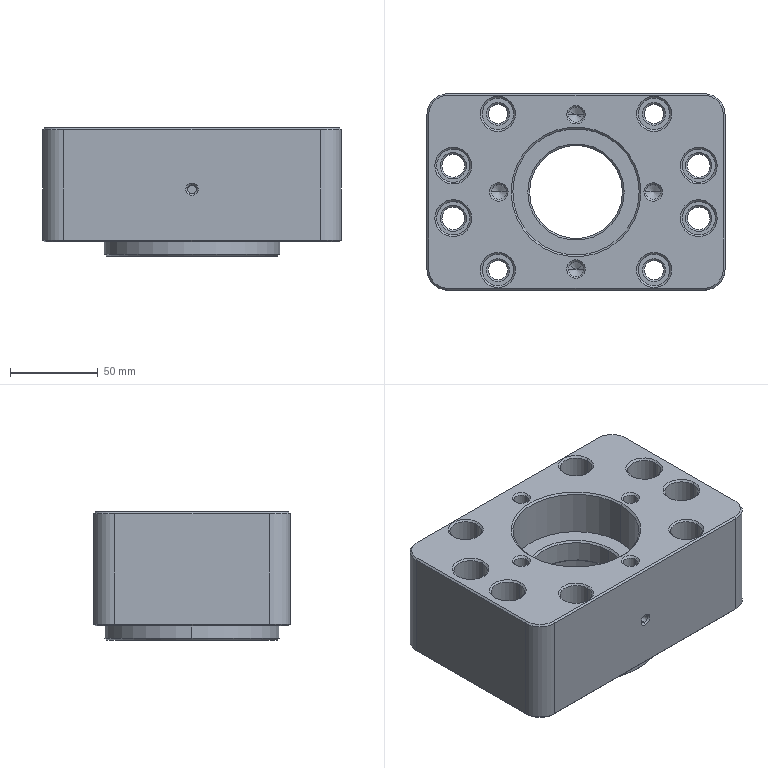NC program | NX | posted with a generic post | part box 170 x 112 x 73 mm
Lines 32 to 1370 of 12427:
(FLOOR_WALL , TOOL : D10C)
N56 T10 M6
N58 G54
N60 G17 G0 G90 X-92. Y28.804 S3500 M3
N62 G43 Z30. H10
N64 Z2.781
N66 G94 G1 Z-0.219 F1000.
N68 X-89.
N70 Y60. F2500.
N72 X89.
N74 Y-60.
N76 X19.577
N78 Y-53.
N80 G3 X19.577 Y53. R56.5
N82 G1 X14.252 Y54.843
N84 X19.577 Y53.
N86 X82.
N88 Y-53.
N90 X43.775
N92 Y-46.
N94 G3 X43.775 Y46. R63.5
N96 G1 X38.884 Y47.847
N98 X43.775 Y46.
N100 X75.
N102 Y18.608
N104 X68.
N106 G3 X58.73 Y39. R70.5
N108 G1 X68.
N110 Y18.608
N112 X67.119 Y13.686
N114 G2 X67.119 Y-13.686 R68.5
N116 X70. Y-14.025 R5.
N118 G1 Y14.025
N120 G2 X67.119 Y13.686 R5.
N122 G1 X68. Y18.608
N124 X75.
N126 Y-46.
N128 X43.775
N130 X38.884 Y-47.847
N132 X43.775 Y-46.
N134 X58.73 Y-39.
N136 G3 X68. Y-18.608 R70.5
N138 G1 Y-39.
N140 X58.73
N142 X43.775 Y-46.
N144 Y-53.
N146 X19.577
N148 X14.252 Y-54.843
N150 X19.577 Y-53.
N152 Y-60.
N154 X-89.
N156 Y28.804
N158 X-82.
N160 Y53.
N162 X-19.577
N164 X-14.252 Y54.843
N166 X-19.577 Y53.
N168 G3 X-19.577 Y-53. R56.5
N170 G1 X-14.252 Y-54.843
N172 X-19.577 Y-53.
N174 X-19.092 Y-51.687
N176 G2 X-51.687 Y19.092 R55.1
N178 X-19.092 Y-51.687 R-55.1
N180 G1 X-19.577 Y-53.
N182 X-82.
N184 Y28.804
N186 X-75.
N188 Y46.
N190 X-43.775
N192 X-38.884 Y47.847
N194 X-43.775 Y46.
N196 G3 X-43.775 Y-46. R63.5
N198 G1 X-38.884 Y-47.847
N200 X-43.775 Y-46.
N202 X-75.
N204 Y-18.608
N206 X-68.
N208 G3 X-58.73 Y-39. R70.5
N210 G1 X-68.
N212 Y-18.608
N214 X-75.
N216 Y28.804
N218 X-68.
N220 Y39.
N222 X-58.73
N224 G3 X-68. Y18.608 R70.5
N226 G1 X-70. Y14.025
N228 Y-14.025
N230 G2 X-67.119 Y-13.686 R5.
N232 X-67.119 Y13.686 R68.5
N234 X-70. Y14.025 R5.
N236 G1 X-68. Y18.608
N238 Y28.804
N240 X-71.
N242 Z2.781
N244 G0 Z30.
N246 X-92.
N248 Z2.561
N250 G1 Z-0.439 F1000.
N252 X-89.
N254 Y60. F2500.
N256 X89.
N258 Y-60.
N260 X19.577
N262 Y-53.
N264 G3 X19.577 Y53. R56.5
N266 G1 X14.252 Y54.843
N268 X19.577 Y53.
N270 X82.
N272 Y-53.
N274 X43.775
N276 Y-46.
N278 G3 X43.775 Y46. R63.5
N280 G1 X38.884 Y47.847
N282 X43.775 Y46.
N284 X75.
N286 Y18.608
N288 X68.
N290 G3 X58.73 Y39. R70.5
N292 G1 X68.
N294 Y18.608
N296 X67.119 Y13.686
N298 G2 X67.119 Y-13.686 R68.5
N300 X70. Y-14.025 R5.
N302 G1 Y14.025
N304 G2 X67.119 Y13.686 R5.
N306 G1 X68. Y18.608
N308 X75.
N310 Y-46.
N312 X43.775
N314 X38.884 Y-47.847
N316 X43.775 Y-46.
N318 X58.73 Y-39.
N320 G3 X68. Y-18.608 R70.5
N322 G1 Y-39.
N324 X58.73
N326 X43.775 Y-46.
N328 Y-53.
N330 X19.577
N332 X14.252 Y-54.843
N334 X19.577 Y-53.
N336 Y-60.
N338 X-89.
N340 Y28.804
N342 X-82.
N344 Y53.
N346 X-19.577
N348 X-14.252 Y54.843
N350 X-19.577 Y53.
N352 G3 X-19.577 Y-53. R56.5
N354 G1 X-14.252 Y-54.843
N356 X-19.577 Y-53.
N358 X-19.092 Y-51.687
N360 G2 X-51.687 Y19.092 R55.1
N362 X-19.092 Y-51.687 R-55.1
N364 G1 X-19.577 Y-53.
N366 X-82.
N368 Y28.804
N370 X-75.
N372 Y46.
N374 X-43.775
N376 X-38.884 Y47.847
N378 X-43.775 Y46.
N380 G3 X-43.775 Y-46. R63.5
N382 G1 X-38.884 Y-47.847
N384 X-43.775 Y-46.
N386 X-75.
N388 Y-18.608
N390 X-68.
N392 G3 X-58.73 Y-39. R70.5
N394 G1 X-68.
N396 Y-18.608
N398 X-75.
N400 Y28.804
N402 X-68.
N404 Y39.
N406 X-58.73
N408 G3 X-68. Y18.608 R70.5
N410 G1 X-70. Y14.025
N412 Y-14.025
N414 G2 X-67.119 Y-13.686 R5.
N416 X-67.119 Y13.686 R68.5
N418 X-70. Y14.025 R5.
N420 G1 X-68. Y18.608
N422 Y28.804
N424 X-71.
N426 Z2.561
N428 G0 Z30.
N430 X-92.
N432 Z2.342
N434 G1 Z-0.658 F1000.
N436 X-89.
N438 Y60. F2500.
N440 X89.
N442 Y-60.
N444 X19.577
N446 Y-53.
N448 G3 X19.577 Y53. R56.5
N450 G1 X14.252 Y54.843
N452 X19.577 Y53.
N454 X82.
N456 Y-53.
N458 X43.775
N460 Y-46.
N462 G3 X43.775 Y46. R63.5
N464 G1 X38.884 Y47.847
N466 X43.775 Y46.
N468 X75.
N470 Y18.608
N472 X68.
N474 G3 X58.73 Y39. R70.5
N476 G1 X68.
N478 Y18.608
N480 X67.119 Y13.686
N482 G2 X67.119 Y-13.686 R68.5
N484 X70. Y-14.025 R5.
N486 G1 Y14.025
N488 G2 X67.119 Y13.686 R5.
N490 G1 X68. Y18.608
N492 X75.
N494 Y-46.
N496 X43.775
N498 X38.884 Y-47.847
N500 X43.775 Y-46.
N502 X58.73 Y-39.
N504 G3 X68. Y-18.608 R70.5
N506 G1 Y-39.
N508 X58.73
N510 X43.775 Y-46.
N512 Y-53.
N514 X19.577
N516 X14.252 Y-54.843
N518 X19.577 Y-53.
N520 Y-60.
N522 X-89.
N524 Y28.804
N526 X-82.
N528 Y53.
N530 X-19.577
N532 X-14.252 Y54.843
N534 X-19.577 Y53.
N536 G3 X-19.577 Y-53. R56.5
N538 G1 X-14.252 Y-54.843
N540 X-19.577 Y-53.
N542 X-19.092 Y-51.687
N544 G2 X-51.687 Y19.092 R55.1
N546 X-19.092 Y-51.687 R-55.1
N548 G1 X-19.577 Y-53.
N550 X-82.
N552 Y28.804
N554 X-75.
N556 Y46.
N558 X-43.775
N560 X-38.884 Y47.847
N562 X-43.775 Y46.
N564 G3 X-43.775 Y-46. R63.5
N566 G1 X-38.884 Y-47.847
N568 X-43.775 Y-46.
N570 X-75.
N572 Y-18.608
N574 X-68.
N576 G3 X-58.73 Y-39. R70.5
N578 G1 X-68.
N580 Y-18.608
N582 X-75.
N584 Y28.804
N586 X-68.
N588 Y39.
N590 X-58.73
N592 G3 X-68. Y18.608 R70.5
N594 G1 X-70. Y14.025
N596 Y-14.025
N598 G2 X-67.119 Y-13.686 R5.
N600 X-67.119 Y13.686 R68.5
N602 X-70. Y14.025 R5.
N604 G1 X-68. Y18.608
N606 Y28.804
N608 X-71.
N610 Z2.342
N612 G0 Z30.
N614 X-92.
N616 Z2.122
N618 G1 Z-0.878 F1000.
N620 X-89.
N622 Y60. F2500.
N624 X89.
N626 Y-60.
N628 X19.577
N630 Y-53.
N632 G3 X19.577 Y53. R56.5
N634 G1 X14.252 Y54.843
N636 X19.577 Y53.
N638 X82.
N640 Y-53.
N642 X43.775
N644 Y-46.
N646 G3 X43.775 Y46. R63.5
N648 G1 X38.884 Y47.847
N650 X43.775 Y46.
N652 X75.
N654 Y18.608
N656 X68.
N658 G3 X58.73 Y39. R70.5
N660 G1 X68.
N662 Y18.608
N664 X67.119 Y13.686
N666 G2 X67.119 Y-13.686 R68.5
N668 X70. Y-14.025 R5.
N670 G1 Y14.025
N672 G2 X67.119 Y13.686 R5.
N674 G1 X68. Y18.608
N676 X75.
N678 Y-46.
N680 X43.775
N682 X38.884 Y-47.847
N684 X43.775 Y-46.
N686 X58.73 Y-39.
N688 G3 X68. Y-18.608 R70.5
N690 G1 Y-39.
N692 X58.73
N694 X43.775 Y-46.
N696 Y-53.
N698 X19.577
N700 X14.252 Y-54.843
N702 X19.577 Y-53.
N704 Y-60.
N706 X-89.
N708 Y28.804
N710 X-82.
N712 Y53.
N714 X-19.577
N716 X-14.252 Y54.843
N718 X-19.577 Y53.
N720 G3 X-19.577 Y-53. R56.5
N722 G1 X-14.252 Y-54.843
N724 X-19.577 Y-53.
N726 X-19.092 Y-51.687
N728 G2 X-51.687 Y19.092 R55.1
N730 X-19.092 Y-51.687 R-55.1
N732 G1 X-19.577 Y-53.
N734 X-82.
N736 Y28.804
N738 X-75.
N740 Y46.
N742 X-43.775
N744 X-38.884 Y47.847
N746 X-43.775 Y46.
N748 G3 X-43.775 Y-46. R63.5
N750 G1 X-38.884 Y-47.847
N752 X-43.775 Y-46.
N754 X-75.
N756 Y-18.608
N758 X-68.
N760 G3 X-58.73 Y-39. R70.5
N762 G1 X-68.
N764 Y-18.608
N766 X-75.
N768 Y28.804
N770 X-68.
N772 Y39.
N774 X-58.73
N776 G3 X-68. Y18.608 R70.5
N778 G1 X-70. Y14.025
N780 Y-14.025
N782 G2 X-67.119 Y-13.686 R5.
N784 X-67.119 Y13.686 R68.5
N786 X-70. Y14.025 R5.
N788 G1 X-68. Y18.608
N790 Y28.804
N792 X-71.
N794 Z2.122
N796 G0 Z30.
N798 X-92.
N800 Z1.903
N802 G1 Z-1.097 F1000.
N804 X-89.
N806 Y60. F2500.
N808 X89.
N810 Y-60.
N812 X19.577
N814 Y-53.
N816 G3 X19.577 Y53. R56.5
N818 G1 X14.252 Y54.843
N820 X19.577 Y53.
N822 X82.
N824 Y-53.
N826 X43.775
N828 Y-46.
N830 G3 X43.775 Y46. R63.5
N832 G1 X38.884 Y47.847
N834 X43.775 Y46.
N836 X75.
N838 Y18.608
N840 X68.
N842 G3 X58.73 Y39. R70.5
N844 G1 X68.
N846 Y18.608
N848 X67.119 Y13.686
N850 G2 X67.119 Y-13.686 R68.5
N852 X70. Y-14.025 R5.
N854 G1 Y14.025
N856 G2 X67.119 Y13.686 R5.
N858 G1 X68. Y18.608
N860 X75.
N862 Y-46.
N864 X43.775
N866 X38.884 Y-47.847
N868 X43.775 Y-46.
N870 X58.73 Y-39.
N872 G3 X68. Y-18.608 R70.5
N874 G1 Y-39.
N876 X58.73
N878 X43.775 Y-46.
N880 Y-53.
N882 X19.577
N884 X14.252 Y-54.843
N886 X19.577 Y-53.
N888 Y-60.
N890 X-89.
N892 Y28.804
N894 X-82.
N896 Y53.
N898 X-19.577
N900 X-14.252 Y54.843
N902 X-19.577 Y53.
N904 G3 X-19.577 Y-53. R56.5
N906 G1 X-14.252 Y-54.843
N908 X-19.577 Y-53.
N910 X-19.092 Y-51.687
N912 G2 X-51.687 Y19.092 R55.1
N914 X-19.092 Y-51.687 R-55.1
N916 G1 X-19.577 Y-53.
N918 X-82.
N920 Y28.804
N922 X-75.
N924 Y46.
N926 X-43.775
N928 X-38.884 Y47.847
N930 X-43.775 Y46.
N932 G3 X-43.775 Y-46. R63.5
N934 G1 X-38.884 Y-47.847
N936 X-43.775 Y-46.
N938 X-75.
N940 Y-18.608
N942 X-68.
N944 G3 X-58.73 Y-39. R70.5
N946 G1 X-68.
N948 Y-18.608
N950 X-75.
N952 Y28.804
N954 X-68.
N956 Y39.
N958 X-58.73
N960 G3 X-68. Y18.608 R70.5
N962 G1 X-70. Y14.025
N964 Y-14.025
N966 G2 X-67.119 Y-13.686 R5.
N968 X-67.119 Y13.686 R68.5
N970 X-70. Y14.025 R5.
N972 G1 X-68. Y18.608
N974 Y28.804
N976 X-71.
N978 Z1.903
N980 G0 Z30.
N982 X-92.
N984 Z1.683
N986 G1 Z-1.317 F1000.
N988 X-89.
N990 Y60. F2500.
N992 X89.
N994 Y-60.
N996 X19.577
N998 Y-53.
N1000 G3 X19.577 Y53. R56.5
N1002 G1 X14.252 Y54.843
N1004 X19.577 Y53.
N1006 X82.
N1008 Y-53.
N1010 X43.775
N1012 Y-46.
N1014 G3 X43.775 Y46. R63.5
N1016 G1 X38.884 Y47.847
N1018 X43.775 Y46.
N1020 X75.
N1022 Y18.608
N1024 X68.
N1026 G3 X58.73 Y39. R70.5
N1028 G1 X68.
N1030 Y18.608
N1032 X67.119 Y13.686
N1034 G2 X67.119 Y-13.686 R68.5
N1036 X70. Y-14.025 R5.
N1038 G1 Y14.025
N1040 G2 X67.119 Y13.686 R5.
N1042 G1 X68. Y18.608
N1044 X75.
N1046 Y-46.
N1048 X43.775
N1050 X38.884 Y-47.847
N1052 X43.775 Y-46.
N1054 X58.73 Y-39.
N1056 G3 X68. Y-18.608 R70.5
N1058 G1 Y-39.
N1060 X58.73
N1062 X43.775 Y-46.
N1064 Y-53.
N1066 X19.577
N1068 X14.252 Y-54.843
N1070 X19.577 Y-53.
N1072 Y-60.
N1074 X-89.
N1076 Y28.804
N1078 X-82.
N1080 Y53.
N1082 X-19.577
N1084 X-14.252 Y54.843
N1086 X-19.577 Y53.
N1088 G3 X-19.577 Y-53. R56.5
N1090 G1 X-14.252 Y-54.843
N1092 X-19.577 Y-53.
N1094 X-19.092 Y-51.687
N1096 G2 X-51.687 Y19.092 R55.1
N1098 X-19.092 Y-51.687 R-55.1
N1100 G1 X-19.577 Y-53.
N1102 X-82.
N1104 Y28.804
N1106 X-75.
N1108 Y46.
N1110 X-43.775
N1112 X-38.884 Y47.847
N1114 X-43.775 Y46.
N1116 G3 X-43.775 Y-46. R63.5
N1118 G1 X-38.884 Y-47.847
N1120 X-43.775 Y-46.
N1122 X-75.
N1124 Y-18.608
N1126 X-68.
N1128 G3 X-58.73 Y-39. R70.5
N1130 G1 X-68.
N1132 Y-18.608
N1134 X-75.
N1136 Y28.804
N1138 X-68.
N1140 Y39.
N1142 X-58.73
N1144 G3 X-68. Y18.608 R70.5
N1146 G1 X-70. Y14.025
N1148 Y-14.025
N1150 G2 X-67.119 Y-13.686 R5.
N1152 X-67.119 Y13.686 R68.5
N1154 X-70. Y14.025 R5.
N1156 G1 X-68. Y18.608
N1158 Y28.804
N1160 X-71.
N1162 Z1.683
N1164 G0 Z30.
N1166 X-92.
N1168 Z1.464
N1170 G1 Z-1.536 F1000.
N1172 X-89.
N1174 Y60. F2500.
N1176 X89.
N1178 Y-60.
N1180 X19.577
N1182 Y-53.
N1184 G3 X19.577 Y53. R56.5
N1186 G1 X14.252 Y54.843
N1188 X19.577 Y53.
N1190 X82.
N1192 Y-53.
N1194 X43.775
N1196 Y-46.
N1198 G3 X43.775 Y46. R63.5
N1200 G1 X38.884 Y47.847
N1202 X43.775 Y46.
N1204 X75.
N1206 Y18.608
N1208 X68.
N1210 G3 X58.73 Y39. R70.5
N1212 G1 X68.
N1214 Y18.608
N1216 X67.119 Y13.686
N1218 G2 X67.119 Y-13.686 R68.5
N1220 X70. Y-14.025 R5.
N1222 G1 Y14.025
N1224 G2 X67.119 Y13.686 R5.
N1226 G1 X68. Y18.608
N1228 X75.
N1230 Y-46.
N1232 X43.775
N1234 X38.884 Y-47.847
N1236 X43.775 Y-46.
N1238 X58.73 Y-39.
N1240 G3 X68. Y-18.608 R70.5
N1242 G1 Y-39.
N1244 X58.73
N1246 X43.775 Y-46.
N1248 Y-53.
N1250 X19.577
N1252 X14.252 Y-54.843
N1254 X19.577 Y-53.
N1256 Y-60.
N1258 X-89.
N1260 Y28.804
N1262 X-82.
N1264 Y53.
N1266 X-19.577
N1268 X-14.252 Y54.843
N1270 X-19.577 Y53.
N1272 G3 X-19.577 Y-53. R56.5
N1274 G1 X-14.252 Y-54.843
N1276 X-19.577 Y-53.
N1278 X-19.092 Y-51.687
N1280 G2 X-51.687 Y19.092 R55.1
N1282 X-19.092 Y-51.687 R-55.1
N1284 G1 X-19.577 Y-53.
N1286 X-82.
N1288 Y28.804
N1290 X-75.
N1292 Y46.
N1294 X-43.775
N1296 X-38.884 Y47.847
N1298 X-43.775 Y46.
N1300 G3 X-43.775 Y-46. R63.5
N1302 G1 X-38.884 Y-47.847
N1304 X-43.775 Y-46.
N1306 X-75.
N1308 Y-18.608
N1310 X-68.
N1312 G3 X-58.73 Y-39. R70.5
N1314 G1 X-68.
N1316 Y-18.608
N1318 X-75.
N1320 Y28.804
N1322 X-68.
N1324 Y39.
N1326 X-58.73
N1328 G3 X-68. Y18.608 R70.5
N1330 G1 X-70. Y14.025
N1332 Y-14.025
N1334 G2 X-67.119 Y-13.686 R5.
N1336 X-67.119 Y13.686 R68.5
N1338 X-70. Y14.025 R5.
N1340 G1 X-68. Y18.608
N1342 Y28.804
N1344 X-71.
N1346 Z1.464
N1348 G0 Z30.
N1350 X-92.
N1352 Z1.244
N1354 G1 Z-1.756 F1000.
N1356 X-89.
N1358 Y60. F2500.
N1360 X89.
N1362 Y-60.
N1364 X19.577
N1366 Y-53.
N1368 G3 X19.577 Y53. R56.5
N1370 G1 X14.252 Y54.843
N1372 X19.577 Y53.
N1374 X82.
N1376 Y-53.
N1378 X43.775
N1380 Y-46.
N1382 G3 X43.775 Y46. R63.5
N1384 G1 X38.884 Y47.847
N1386 X43.775 Y46.
N1388 X75.
N1390 Y18.608
N1392 X68.
N1394 G3 X58.73 Y39. R70.5
N1396 G1 X68.
N1398 Y18.608
N1400 X67.119 Y13.686
N1402 G2 X67.119 Y-13.686 R68.5
N1404 X70. Y-14.025 R5.
N1406 G1 Y14.025
N1408 G2 X67.119 Y13.686 R5.
N1410 G1 X68. Y18.608
N1412 X75.
N1414 Y-46.
N1416 X43.775
N1418 X38.884 Y-47.847
N1420 X43.775 Y-46.
N1422 X58.73 Y-39.
N1424 G3 X68. Y-18.608 R70.5
N1426 G1 Y-39.
N1428 X58.73
N1430 X43.775 Y-46.
N1432 Y-53.
N1434 X19.577
N1436 X14.252 Y-54.843
N1438 X19.577 Y-53.
N1440 Y-60.
N1442 X-89.
N1444 Y28.804
N1446 X-82.
N1448 Y53.
N1450 X-19.577
N1452 X-14.252 Y54.843
N1454 X-19.577 Y53.
N1456 G3 X-19.577 Y-53. R56.5
N1458 G1 X-14.252 Y-54.843
N1460 X-19.577 Y-53.
N1462 X-19.092 Y-51.687
N1464 G2 X-51.687 Y19.092 R55.1
N1466 X-19.092 Y-51.687 R-55.1
N1468 G1 X-19.577 Y-53.
N1470 X-82.
N1472 Y28.804
N1474 X-75.
N1476 Y46.
N1478 X-43.775
N1480 X-38.884 Y47.847
N1482 X-43.775 Y46.
N1484 G3 X-43.775 Y-46. R63.5
N1486 G1 X-38.884 Y-47.847
N1488 X-43.775 Y-46.
N1490 X-75.
N1492 Y-18.608
N1494 X-68.
N1496 G3 X-58.73 Y-39. R70.5
N1498 G1 X-68.
N1500 Y-18.608
N1502 X-75.
N1504 Y28.804
N1506 X-68.
N1508 Y39.
N1510 X-58.73
N1512 G3 X-68. Y18.608 R70.5
N1514 G1 X-70. Y14.025
N1516 Y-14.025
N1518 G2 X-67.119 Y-13.686 R5.
N1520 X-67.119 Y13.686 R68.5
N1522 X-70. Y14.025 R5.
N1524 G1 X-68. Y18.608
N1526 Y28.804
N1528 X-71.
N1530 Z1.244
N1532 G0 Z30.
N1534 X-92.
N1536 Z1.025
N1538 G1 Z-1.975 F1000.
N1540 X-89.
N1542 Y60. F2500.
N1544 X89.
N1546 Y-60.
N1548 X19.577
N1550 Y-53.
N1552 G3 X19.577 Y53. R56.5
N1554 G1 X14.252 Y54.843
N1556 X19.577 Y53.
N1558 X82.
N1560 Y-53.
N1562 X43.775
N1564 Y-46.
N1566 G3 X43.775 Y46. R63.5
N1568 G1 X38.884 Y47.847
N1570 X43.775 Y46.
N1572 X75.
N1574 Y18.608
N1576 X68.
N1578 G3 X58.73 Y39. R70.5
N1580 G1 X68.
N1582 Y18.608
N1584 X67.119 Y13.686
N1586 G2 X67.119 Y-13.686 R68.5
N1588 X70. Y-14.025 R5.
N1590 G1 Y14.025
N1592 G2 X67.119 Y13.686 R5.
N1594 G1 X68. Y18.608
N1596 X75.
N1598 Y-46.
N1600 X43.775
N1602 X38.884 Y-47.847
N1604 X43.775 Y-46.
N1606 X58.73 Y-39.
N1608 G3 X68. Y-18.608 R70.5
N1610 G1 Y-39.
N1612 X58.73
N1614 X43.775 Y-46.
N1616 Y-53.
N1618 X19.577
N1620 X14.252 Y-54.843
N1622 X19.577 Y-53.
N1624 Y-60.
N1626 X-89.
N1628 Y28.804
N1630 X-82.
N1632 Y53.
N1634 X-19.577
N1636 X-14.252 Y54.843
N1638 X-19.577 Y53.
N1640 G3 X-19.577 Y-53. R56.5
N1642 G1 X-14.252 Y-54.843
N1644 X-19.577 Y-53.
N1646 X-19.092 Y-51.687
N1648 G2 X-51.687 Y19.092 R55.1
N1650 X-19.092 Y-51.687 R-55.1
N1652 G1 X-19.577 Y-53.
N1654 X-82.
N1656 Y28.804
N1658 X-75.
N1660 Y46.
N1662 X-43.775
N1664 X-38.884 Y47.847
N1666 X-43.775 Y46.
N1668 G3 X-43.775 Y-46. R63.5
N1670 G1 X-38.884 Y-47.847
N1672 X-43.775 Y-46.
N1674 X-75.
N1676 Y-18.608
N1678 X-68.
N1680 G3 X-58.73 Y-39. R70.5
N1682 G1 X-68.
N1684 Y-18.608
N1686 X-75.
N1688 Y28.804
N1690 X-68.
N1692 Y39.
N1694 X-58.73
N1696 G3 X-68. Y18.608 R70.5
N1698 G1 X-70. Y14.025
N1700 Y-14.025
N1702 G2 X-67.119 Y-13.686 R5.
N1704 X-67.119 Y13.686 R68.5
N1706 X-70. Y14.025 R5.
N1708 G1 X-68. Y18.608
N1710 Y28.804
N1712 X-71.
N1714 Z1.025
N1716 G0 Z30.
N1718 X-92.
N1720 Z0.806
N1722 G1 Z-2.194 F1000.
N1724 X-89.
N1726 Y60. F2500.
N1728 X89.
N1730 Y-60.
N1732 X19.577
N1734 Y-53.
N1736 G3 X19.577 Y53. R56.5
N1738 G1 X14.252 Y54.843
N1740 X19.577 Y53.
N1742 X82.
N1744 Y-53.
N1746 X43.775
N1748 Y-46.
N1750 G3 X43.775 Y46. R63.5
N1752 G1 X38.884 Y47.847
N1754 X43.775 Y46.
N1756 X75.
N1758 Y18.608
N1760 X68.
N1762 G3 X58.73 Y39. R70.5
N1764 G1 X68.
N1766 Y18.608
N1768 X67.119 Y13.686
N1770 G2 X67.119 Y-13.686 R68.5
N1772 X70. Y-14.025 R5.
N1774 G1 Y14.025
N1776 G2 X67.119 Y13.686 R5.
N1778 G1 X68. Y18.608
N1780 X75.
N1782 Y-46.
N1784 X43.775
N1786 X38.884 Y-47.847
N1788 X43.775 Y-46.
N1790 X58.73 Y-39.
N1792 G3 X68. Y-18.608 R70.5
N1794 G1 Y-39.
N1796 X58.73
N1798 X43.775 Y-46.
N1800 Y-53.
N1802 X19.577
N1804 X14.252 Y-54.843
N1806 X19.577 Y-53.
N1808 Y-60.
N1810 X-89.
N1812 Y28.804
N1814 X-82.
N1816 Y53.
N1818 X-19.577
N1820 X-14.252 Y54.843
N1822 X-19.577 Y53.
N1824 G3 X-19.577 Y-53. R56.5
N1826 G1 X-14.252 Y-54.843
N1828 X-19.577 Y-53.
N1830 X-19.092 Y-51.687
N1832 G2 X-51.687 Y19.092 R55.1
N1834 X-19.092 Y-51.687 R-55.1
N1836 G1 X-19.577 Y-53.
N1838 X-82.
N1840 Y28.804
N1842 X-75.
N1844 Y46.
N1846 X-43.775
N1848 X-38.884 Y47.847
N1850 X-43.775 Y46.
N1852 G3 X-43.775 Y-46. R63.5
N1854 G1 X-38.884 Y-47.847
N1856 X-43.775 Y-46.
N1858 X-75.
N1860 Y-18.608
N1862 X-68.
N1864 G3 X-58.73 Y-39. R70.5
N1866 G1 X-68.
N1868 Y-18.608
N1870 X-75.
N1872 Y28.804
N1874 X-68.
N1876 Y39.
N1878 X-58.73
N1880 G3 X-68. Y18.608 R70.5
N1882 G1 X-70. Y14.025
N1884 Y-14.025
N1886 G2 X-67.119 Y-13.686 R5.
N1888 X-67.119 Y13.686 R68.5
N1890 X-70. Y14.025 R5.
N1892 G1 X-68. Y18.608
N1894 Y28.804
N1896 X-71.
N1898 Z0.806
N1900 G0 Z30.
N1902 X-92.
N1904 Z0.586
N1906 G1 Z-2.414 F1000.
N1908 X-89.
N1910 Y60. F2500.
N1912 X89.
N1914 Y-60.
N1916 X19.577
N1918 Y-53.
N1920 G3 X19.577 Y53. R56.5
N1922 G1 X14.252 Y54.843
N1924 X19.577 Y53.
N1926 X82.
N1928 Y-53.
N1930 X43.775
N1932 Y-46.
N1934 G3 X43.775 Y46. R63.5
N1936 G1 X38.884 Y47.847
N1938 X43.775 Y46.
N1940 X75.
N1942 Y18.608
N1944 X68.
N1946 G3 X58.73 Y39. R70.5
N1948 G1 X68.
N1950 Y18.608
N1952 X67.119 Y13.686
N1954 G2 X67.119 Y-13.686 R68.5
N1956 X70. Y-14.025 R5.
N1958 G1 Y14.025
N1960 G2 X67.119 Y13.686 R5.
N1962 G1 X68. Y18.608
N1964 X75.
N1966 Y-46.
N1968 X43.775
N1970 X38.884 Y-47.847
N1972 X43.775 Y-46.
N1974 X58.73 Y-39.
N1976 G3 X68. Y-18.608 R70.5
N1978 G1 Y-39.
N1980 X58.73
N1982 X43.775 Y-46.
N1984 Y-53.
N1986 X19.577
N1988 X14.252 Y-54.843
N1990 X19.577 Y-53.
N1992 Y-60.
N1994 X-89.
N1996 Y28.804
N1998 X-82.
N2000 Y53.
N2002 X-19.577
N2004 X-14.252 Y54.843
N2006 X-19.577 Y53.
N2008 G3 X-19.577 Y-53. R56.5
N2010 G1 X-14.252 Y-54.843
N2012 X-19.577 Y-53.
N2014 X-19.092 Y-51.687
N2016 G2 X-51.687 Y19.092 R55.1
N2018 X-19.092 Y-51.687 R-55.1
N2020 G1 X-19.577 Y-53.
N2022 X-82.
N2024 Y28.804
N2026 X-75.
N2028 Y46.
N2030 X-43.775
N2032 X-38.884 Y47.847
N2034 X-43.775 Y46.
N2036 G3 X-43.775 Y-46. R63.5
N2038 G1 X-38.884 Y-47.847
N2040 X-43.775 Y-46.
N2042 X-75.
N2044 Y-18.608
N2046 X-68.
N2048 G3 X-58.73 Y-39. R70.5
N2050 G1 X-68.
N2052 Y-18.608
N2054 X-75.
N2056 Y28.804
N2058 X-68.
N2060 Y39.
N2062 X-58.73
N2064 G3 X-68. Y18.608 R70.5
N2066 G1 X-70. Y14.025
N2068 Y-14.025
N2070 G2 X-67.119 Y-13.686 R5.
N2072 X-67.119 Y13.686 R68.5
N2074 X-70. Y14.025 R5.
N2076 G1 X-68. Y18.608
N2078 Y28.804
N2080 X-71.
N2082 Z0.586
N2084 G0 Z30.
N2086 X-92.
N2088 Z0.367
N2090 G1 Z-2.633 F1000.
N2092 X-89.
N2094 Y60. F2500.
N2096 X89.
N2098 Y-60.
N2100 X19.577
N2102 Y-53.
N2104 G3 X19.577 Y53. R56.5
N2106 G1 X14.252 Y54.843
N2108 X19.577 Y53.
N2110 X82.
N2112 Y-53.
N2114 X43.775
N2116 Y-46.
N2118 G3 X43.775 Y46. R63.5
N2120 G1 X38.884 Y47.847
N2122 X43.775 Y46.
N2124 X75.
N2126 Y18.608
N2128 X68.
N2130 G3 X58.73 Y39. R70.5
N2132 G1 X68.
N2134 Y18.608
N2136 X67.119 Y13.686
N2138 G2 X67.119 Y-13.686 R68.5
N2140 X70. Y-14.025 R5.
N2142 G1 Y14.025
N2144 G2 X67.119 Y13.686 R5.
N2146 G1 X68. Y18.608
N2148 X75.
N2150 Y-46.
N2152 X43.775
N2154 X38.884 Y-47.847
N2156 X43.775 Y-46.
N2158 X58.73 Y-39.
N2160 G3 X68. Y-18.608 R70.5
N2162 G1 Y-39.
N2164 X58.73
N2166 X43.775 Y-46.
N2168 Y-53.
N2170 X19.577
N2172 X14.252 Y-54.843
N2174 X19.577 Y-53.
N2176 Y-60.
N2178 X-89.
N2180 Y28.804
N2182 X-82.
N2184 Y53.
N2186 X-19.577
N2188 X-14.252 Y54.843
N2190 X-19.577 Y53.
N2192 G3 X-19.577 Y-53. R56.5
N2194 G1 X-14.252 Y-54.843
N2196 X-19.577 Y-53.
N2198 X-19.092 Y-51.687
N2200 G2 X-51.687 Y19.092 R55.1
N2202 X-19.092 Y-51.687 R-55.1
N2204 G1 X-19.577 Y-53.
N2206 X-82.
N2208 Y28.804
N2210 X-75.
N2212 Y46.
N2214 X-43.775
N2216 X-38.884 Y47.847
N2218 X-43.775 Y46.
N2220 G3 X-43.775 Y-46. R63.5
N2222 G1 X-38.884 Y-47.847
N2224 X-43.775 Y-46.
N2226 X-75.
N2228 Y-18.608
N2230 X-68.
N2232 G3 X-58.73 Y-39. R70.5
N2234 G1 X-68.
N2236 Y-18.608
N2238 X-75.
N2240 Y28.804
N2242 X-68.
N2244 Y39.
N2246 X-58.73
N2248 G3 X-68. Y18.608 R70.5
N2250 G1 X-70. Y14.025
N2252 Y-14.025
N2254 G2 X-67.119 Y-13.686 R5.
N2256 X-67.119 Y13.686 R68.5
N2258 X-70. Y14.025 R5.
N2260 G1 X-68. Y18.608
N2262 Y28.804
N2264 X-71.
N2266 Z0.367
N2268 G0 Z30.
N2270 X-92.
N2272 Z0.147
N2274 G1 Z-2.853 F1000.
N2276 X-89.
N2278 Y60. F2500.
N2280 X89.
N2282 Y-60.
N2284 X19.577
N2286 Y-53.
N2288 G3 X19.577 Y53. R56.5
N2290 G1 X14.252 Y54.843
N2292 X19.577 Y53.
N2294 X82.
N2296 Y-53.
N2298 X43.775
N2300 Y-46.
N2302 G3 X43.775 Y46. R63.5
N2304 G1 X38.884 Y47.847
N2306 X43.775 Y46.
N2308 X75.
N2310 Y18.608
N2312 X68.
N2314 G3 X58.73 Y39. R70.5
N2316 G1 X68.
N2318 Y18.608
N2320 X67.119 Y13.686
N2322 G2 X67.119 Y-13.686 R68.5
N2324 X70. Y-14.025 R5.
N2326 G1 Y14.025
N2328 G2 X67.119 Y13.686 R5.
N2330 G1 X68. Y18.608
N2332 X75.
N2334 Y-46.
N2336 X43.775
N2338 X38.884 Y-47.847
N2340 X43.775 Y-46.
N2342 X58.73 Y-39.
N2344 G3 X68. Y-18.608 R70.5
N2346 G1 Y-39.
N2348 X58.73
N2350 X43.775 Y-46.
N2352 Y-53.
N2354 X19.577
N2356 X14.252 Y-54.843
N2358 X19.577 Y-53.
N2360 Y-60.
N2362 X-89.
N2364 Y28.804
N2366 X-82.
N2368 Y53.
N2370 X-19.577
N2372 X-14.252 Y54.843
N2374 X-19.577 Y53.
N2376 G3 X-19.577 Y-53. R56.5
N2378 G1 X-14.252 Y-54.843
N2380 X-19.577 Y-53.
N2382 X-19.092 Y-51.687
N2384 G2 X-51.687 Y19.092 R55.1
N2386 X-19.092 Y-51.687 R-55.1
N2388 G1 X-19.577 Y-53.
N2390 X-82.
N2392 Y28.804
N2394 X-75.
N2396 Y46.
N2398 X-43.775
N2400 X-38.884 Y47.847
N2402 X-43.775 Y46.
N2404 G3 X-43.775 Y-46. R63.5
N2406 G1 X-38.884 Y-47.847
N2408 X-43.775 Y-46.
N2410 X-75.
N2412 Y-18.608
N2414 X-68.
N2416 G3 X-58.73 Y-39. R70.5
N2418 G1 X-68.
N2420 Y-18.608
N2422 X-75.
N2424 Y28.804
N2426 X-68.
N2428 Y39.
N2430 X-58.73
N2432 G3 X-68. Y18.608 R70.5
N2434 G1 X-70. Y14.025
N2436 Y-14.025
N2438 G2 X-67.119 Y-13.686 R5.
N2440 X-67.119 Y13.686 R68.5
N2442 X-70. Y14.025 R5.
N2444 G1 X-68. Y18.608
N2446 Y28.804
N2448 X-71.
N2450 Z0.147
N2452 G0 Z30.
N2454 X-92.
N2456 Z-0.072
N2458 G1 Z-3.072 F1000.
N2460 X-89.
N2462 Y60. F2500.
N2464 X89.
N2466 Y-60.
N2468 X19.577
N2470 Y-53.
N2472 G3 X19.577 Y53. R56.5
N2474 G1 X14.252 Y54.843
N2476 X19.577 Y53.
N2478 X82.
N2480 Y-53.
N2482 X43.775
N2484 Y-46.
N2486 G3 X43.775 Y46. R63.5
N2488 G1 X38.884 Y47.847
N2490 X43.775 Y46.
N2492 X75.
N2494 Y18.608
N2496 X68.
N2498 G3 X58.73 Y39. R70.5
N2500 G1 X68.
N2502 Y18.608
N2504 X67.119 Y13.686
N2506 G2 X67.119 Y-13.686 R68.5
N2508 X70. Y-14.025 R5.
N2510 G1 Y14.025
N2512 G2 X67.119 Y13.686 R5.
N2514 G1 X68. Y18.608
N2516 X75.
N2518 Y-46.
N2520 X43.775
N2522 X38.884 Y-47.847
N2524 X43.775 Y-46.
N2526 X58.73 Y-39.
N2528 G3 X68. Y-18.608 R70.5
N2530 G1 Y-39.
N2532 X58.73
N2534 X43.775 Y-46.
N2536 Y-53.
N2538 X19.577
N2540 X14.252 Y-54.843
N2542 X19.577 Y-53.
N2544 Y-60.
N2546 X-89.
N2548 Y28.804
N2550 X-82.
N2552 Y53.
N2554 X-19.577
N2556 X-14.252 Y54.843
N2558 X-19.577 Y53.
N2560 G3 X-19.577 Y-53. R56.5
N2562 G1 X-14.252 Y-54.843
N2564 X-19.577 Y-53.
N2566 X-19.092 Y-51.687
N2568 G2 X-51.687 Y19.092 R55.1
N2570 X-19.092 Y-51.687 R-55.1
N2572 G1 X-19.577 Y-53.
N2574 X-82.
N2576 Y28.804
N2578 X-75.
N2580 Y46.
N2582 X-43.775
N2584 X-38.884 Y47.847
N2586 X-43.775 Y46.
N2588 G3 X-43.775 Y-46. R63.5
N2590 G1 X-38.884 Y-47.847
N2592 X-43.775 Y-46.
N2594 X-75.
N2596 Y-18.608
N2598 X-68.
N2600 G3 X-58.73 Y-39. R70.5
N2602 G1 X-68.
N2604 Y-18.608
N2606 X-75.
N2608 Y28.804
N2610 X-68.
N2612 Y39.
N2614 X-58.73
N2616 G3 X-68. Y18.608 R70.5
N2618 G1 X-70. Y14.025
N2620 Y-14.025
N2622 G2 X-67.119 Y-13.686 R5.
N2624 X-67.119 Y13.686 R68.5
N2626 X-70. Y14.025 R5.
N2628 G1 X-68. Y18.608
N2630 Y28.804
N2632 X-71.
N2634 Z-0.072
N2636 G0 Z30.
N2638 X-92.
N2640 Z-0.292
N2642 G1 Z-3.292 F1000.
N2644 X-89.
N2646 Y60. F2500.
N2648 X89.
N2650 Y-60.
N2652 X19.577
N2654 Y-53.
N2656 G3 X19.577 Y53. R56.5
N2658 G1 X14.252 Y54.843
N2660 X19.577 Y53.
N2662 X82.
N2664 Y-53.
N2666 X43.775
N2668 Y-46.
N2670 G3 X43.775 Y46. R63.5
N2672 G1 X38.884 Y47.847
N2674 X43.775 Y46.
N2676 X75.
N2678 Y18.608
N2680 X68.
N2682 G3 X58.73 Y39. R70.5
N2684 G1 X68.
N2686 Y18.608
N2688 X67.119 Y13.686
N2690 G2 X67.119 Y-13.686 R68.5
N2692 X70. Y-14.025 R5.
N2694 G1 Y14.025
N2696 G2 X67.119 Y13.686 R5.
N2698 G1 X68. Y18.608
N2700 X75.
N2702 Y-46.
N2704 X43.775
N2706 X38.884 Y-47.847
N2708 X43.775 Y-46.
N2710 X58.73 Y-39.
N2712 G3 X68. Y-18.608 R70.5
N2714 G1 Y-39.
N2716 X58.73
N2718 X43.775 Y-46.
N2720 Y-53.
N2722 X19.577
N2724 X14.252 Y-54.843
N2726 X19.577 Y-53.